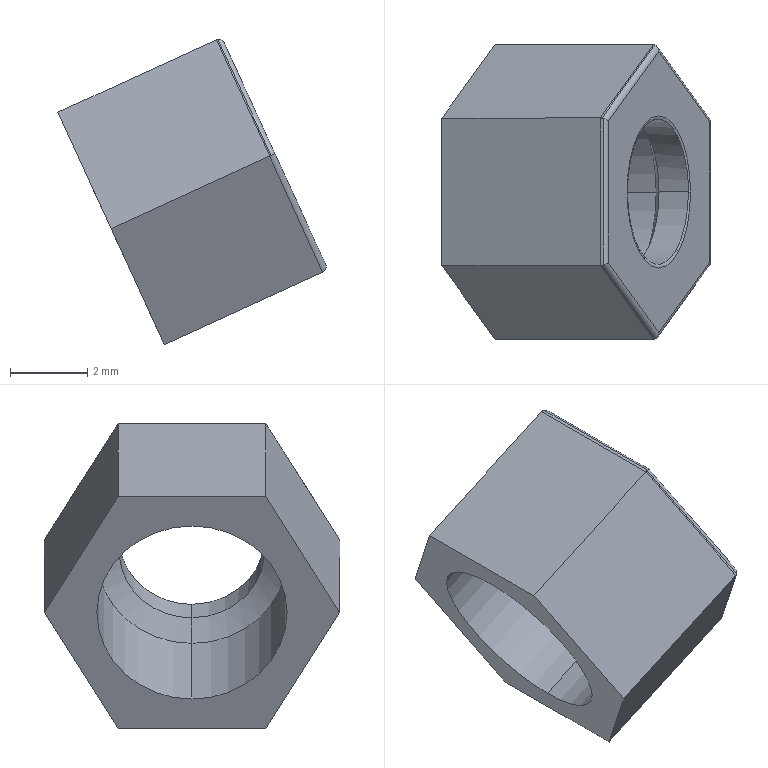Part | STEP file | 2026.6.15-Main Assembly图.sldasm-Part-206 | 1 solid | 25 faces | box 6.927 x 7.621 x 7.888 mm | volume 95.325 mm3 | cylinder 13 | plane 8 | torus 2 | cone 2 | commonest cylinder face diameters 0.3 x9 3.75 x2 4.913 x2
STEP:
#1=CARTESIAN_POINT('',(-1606.587,1438.31,3412.574));
#2=VERTEX_POINT('',#1);
#3=CARTESIAN_POINT('',(-1606.623,1438.304,3412.557));
#4=VERTEX_POINT('',#3);
#5=CARTESIAN_POINT('',(-1606.587,1438.31,3412.574));
#6=CARTESIAN_POINT('',(-1606.599,1438.306,3412.568));
#7=CARTESIAN_POINT('',(-1606.611,1438.304,3412.563));
#8=CARTESIAN_POINT('',(-1606.623,1438.304,3412.557));
#9=(BOUNDED_CURVE()B_SPLINE_CURVE(3,(#5,#6,#7,#8),.UNSPECIFIED.,.F.,.F.)B_SPLINE_CURVE_WITH_KNOTS((4,4),(0.8172,1.),.UNSPECIFIED.)CURVE()GEOMETRIC_REPRESENTATION_ITEM()RATIONAL_B_SPLINE_CURVE((0.9125,0.9351,0.9643,1.))REPRESENTATION_ITEM(''));
#10=EDGE_CURVE('',#2,#4,#9,.T.);
#11=ORIENTED_EDGE('',*,*,#10,.F.);
#12=CARTESIAN_POINT('',(-1607.958,1440.212,3415.569));
#13=VERTEX_POINT('',#12);
#14=CARTESIAN_POINT('',(-1609.333,1442.119,3418.572));
#15=DIRECTION('',(-0.3605,0.5,0.7874));
#16=VECTOR('',#15,1000.);
#17=LINE('',#14,#16);
#18=EDGE_CURVE('',#2,#13,#17,.T.);
#19=ORIENTED_EDGE('',*,*,#18,.T.);
#20=CARTESIAN_POINT('',(-1607.997,1440.209,3415.558));
#21=VERTEX_POINT('',#20);
#22=CARTESIAN_POINT('',(-1607.958,1440.212,3415.569));
#23=CARTESIAN_POINT('',(-1607.972,1440.21,3415.567));
#24=CARTESIAN_POINT('',(-1607.985,1440.209,3415.563));
#25=CARTESIAN_POINT('',(-1607.997,1440.209,3415.558));
#26=(BOUNDED_CURVE()B_SPLINE_CURVE(3,(#22,#23,#24,#25),.UNSPECIFIED.,.F.,.T.)B_SPLINE_CURVE_WITH_KNOTS((4,4),(0.8172,1.),.UNSPECIFIED.)CURVE()GEOMETRIC_REPRESENTATION_ITEM()RATIONAL_B_SPLINE_CURVE((0.9125,0.9351,0.9643,1.))REPRESENTATION_ITEM(''));
#27=EDGE_CURVE('',#13,#21,#26,.T.);
#28=ORIENTED_EDGE('',*,*,#27,.T.);
#29=CARTESIAN_POINT('',(-1606.623,1438.304,3412.557));
#30=DIRECTION('',(-0.3605,0.5,0.7874));
#31=VECTOR('',#30,1000.);
#32=LINE('',#29,#31);
#33=EDGE_CURVE('',#4,#21,#32,.T.);
#34=ORIENTED_EDGE('',*,*,#33,.F.);
#35=EDGE_LOOP('',(#11,#19,#28,#34));
#36=FACE_OUTER_BOUND('',#35,.T.);
#37=CARTESIAN_POINT('',(-1609.339,1442.244,3418.49));
#38=DIRECTION('',(-0.3605,0.5,0.7874));
#39=DIRECTION('',(0.04327,-0.8343,0.5496));
#40=AXIS2_PLACEMENT_3D('',#37,#38,#39);
#41=CYLINDRICAL_SURFACE('',#40,0.15);
#42=ADVANCED_FACE('',(#36),#41,.T.);
#43=CARTESIAN_POINT('',(-1607.923,1440.22,3415.571));
#44=VERTEX_POINT('',#43);
#45=CARTESIAN_POINT('',(-1607.923,1440.22,3415.571));
#46=CARTESIAN_POINT('',(-1607.934,1440.217,3415.572));
#47=CARTESIAN_POINT('',(-1607.946,1440.214,3415.571));
#48=CARTESIAN_POINT('',(-1607.958,1440.212,3415.569));
#49=(BOUNDED_CURVE()B_SPLINE_CURVE(3,(#45,#46,#47,#48),.UNSPECIFIED.,.F.,.T.)B_SPLINE_CURVE_WITH_KNOTS((4,4),(0.6686,0.8172),.UNSPECIFIED.)CURVE()GEOMETRIC_REPRESENTATION_ITEM()RATIONAL_B_SPLINE_CURVE((0.8702,0.88,0.8941,0.9125))REPRESENTATION_ITEM(''));
#50=EDGE_CURVE('',#44,#13,#49,.T.);
#51=ORIENTED_EDGE('',*,*,#50,.F.);
#52=CARTESIAN_POINT('',(-1607.923,1444.009,3415.571));
#53=VERTEX_POINT('',#52);
#54=CARTESIAN_POINT('',(-1607.923,1442.114,3415.571));
#55=DIRECTION('',(0.,1.,0.));
#56=VECTOR('',#55,1000.);
#57=LINE('',#54,#56);
#58=EDGE_CURVE('',#44,#53,#57,.T.);
#59=ORIENTED_EDGE('',*,*,#58,.T.);
#60=CARTESIAN_POINT('',(-1607.958,1444.016,3415.569));
#61=VERTEX_POINT('',#60);
#62=CARTESIAN_POINT('',(-1607.923,1444.009,3415.571));
#63=CARTESIAN_POINT('',(-1607.934,1444.012,3415.572));
#64=CARTESIAN_POINT('',(-1607.946,1444.015,3415.571));
#65=CARTESIAN_POINT('',(-1607.958,1444.016,3415.569));
#66=(BOUNDED_CURVE()B_SPLINE_CURVE(3,(#62,#63,#64,#65),.UNSPECIFIED.,.F.,.F.)B_SPLINE_CURVE_WITH_KNOTS((4,4),(0.6686,0.8172),.UNSPECIFIED.)CURVE()GEOMETRIC_REPRESENTATION_ITEM()RATIONAL_B_SPLINE_CURVE((0.8702,0.88,0.8941,0.9125))REPRESENTATION_ITEM(''));
#67=EDGE_CURVE('',#53,#61,#66,.T.);
#68=ORIENTED_EDGE('',*,*,#67,.T.);
#69=CARTESIAN_POINT('',(-1607.997,1444.02,3415.558));
#70=VERTEX_POINT('',#69);
#71=CARTESIAN_POINT('',(-1607.958,1444.016,3415.569));
#72=CARTESIAN_POINT('',(-1607.972,1444.019,3415.567));
#73=CARTESIAN_POINT('',(-1607.985,1444.02,3415.563));
#74=CARTESIAN_POINT('',(-1607.997,1444.02,3415.558));
#75=(BOUNDED_CURVE()B_SPLINE_CURVE(3,(#71,#72,#73,#74),.UNSPECIFIED.,.F.,.F.)B_SPLINE_CURVE_WITH_KNOTS((4,4),(0.8172,1.),.UNSPECIFIED.)CURVE()GEOMETRIC_REPRESENTATION_ITEM()RATIONAL_B_SPLINE_CURVE((0.9125,0.9351,0.9643,1.))REPRESENTATION_ITEM(''));
#76=EDGE_CURVE('',#61,#70,#75,.T.);
#77=ORIENTED_EDGE('',*,*,#76,.T.);
#78=CARTESIAN_POINT('',(-1607.997,1444.02,3415.558));
#79=DIRECTION('',(0.,1.,0.));
#80=VECTOR('',#79,1000.);
#81=LINE('',#78,#80);
#82=EDGE_CURVE('',#21,#70,#81,.T.);
#83=ORIENTED_EDGE('',*,*,#82,.F.);
#84=ORIENTED_EDGE('',*,*,#27,.F.);
#85=EDGE_LOOP('',(#51,#59,#68,#77,#83,#84));
#86=FACE_OUTER_BOUND('',#85,.T.);
#87=CARTESIAN_POINT('',(-1607.934,1442.114,3415.421));
#88=DIRECTION('',(0.,1.,0.));
#89=DIRECTION('',(0.0785,0.,0.9969));
#90=AXIS2_PLACEMENT_3D('',#87,#88,#89);
#91=CYLINDRICAL_SURFACE('',#90,0.15);
#92=ADVANCED_FACE('',(#86),#91,.T.);
#93=ORIENTED_EDGE('',*,*,#76,.F.);
#94=CARTESIAN_POINT('',(-1606.587,1445.918,3412.574));
#95=VERTEX_POINT('',#94);
#96=CARTESIAN_POINT('',(-1609.333,1442.11,3418.572));
#97=DIRECTION('',(0.3605,0.5,-0.7874));
#98=VECTOR('',#97,1000.);
#99=LINE('',#96,#98);
#100=EDGE_CURVE('',#61,#95,#99,.T.);
#101=ORIENTED_EDGE('',*,*,#100,.T.);
#102=CARTESIAN_POINT('',(-1606.623,1445.925,3412.557));
#103=VERTEX_POINT('',#102);
#104=CARTESIAN_POINT('',(-1606.623,1445.925,3412.557));
#105=CARTESIAN_POINT('',(-1606.611,1445.925,3412.563));
#106=CARTESIAN_POINT('',(-1606.599,1445.923,3412.568));
#107=CARTESIAN_POINT('',(-1606.587,1445.918,3412.574));
#108=(BOUNDED_CURVE()B_SPLINE_CURVE(3,(#104,#105,#106,#107),.UNSPECIFIED.,.F.,.T.)B_SPLINE_CURVE_WITH_KNOTS((4,4),(0.,0.1828),.UNSPECIFIED.)CURVE()GEOMETRIC_REPRESENTATION_ITEM()RATIONAL_B_SPLINE_CURVE((1.,0.9643,0.9351,0.9125))REPRESENTATION_ITEM(''));
#109=EDGE_CURVE('',#103,#95,#108,.T.);
#110=ORIENTED_EDGE('',*,*,#109,.F.);
#111=CARTESIAN_POINT('',(-1607.997,1444.02,3415.558));
#112=DIRECTION('',(0.3605,0.5,-0.7874));
#113=VECTOR('',#112,1000.);
#114=LINE('',#111,#113);
#115=EDGE_CURVE('',#70,#103,#114,.T.);
#116=ORIENTED_EDGE('',*,*,#115,.F.);
#117=EDGE_LOOP('',(#93,#101,#110,#116));
#118=FACE_OUTER_BOUND('',#117,.T.);
#119=CARTESIAN_POINT('',(-1609.339,1441.984,3418.49));
#120=DIRECTION('',(0.3605,0.5,-0.7874));
#121=DIRECTION('',(0.04327,0.8343,0.5496));
#122=AXIS2_PLACEMENT_3D('',#119,#120,#121);
#123=CYLINDRICAL_SURFACE('',#122,0.15);
#124=ADVANCED_FACE('',(#118),#123,.T.);
#125=CARTESIAN_POINT('',(-1605.175,1440.296,3409.756));
#126=VERTEX_POINT('',#125);
#127=CARTESIAN_POINT('',(-1606.487,1438.477,3412.62));
#128=VERTEX_POINT('',#127);
#129=CARTESIAN_POINT('',(-1607.892,1436.528,3415.688));
#130=DIRECTION('',(-0.3605,-0.5,0.7874));
#131=VECTOR('',#130,1000.);
#132=LINE('',#129,#131);
#133=EDGE_CURVE('',#126,#128,#132,.T.);
#134=ORIENTED_EDGE('',*,*,#133,.F.);
#135=CARTESIAN_POINT('',(-1605.175,1443.933,3409.756));
#136=VERTEX_POINT('',#135);
#137=CARTESIAN_POINT('',(-1605.175,1442.114,3409.756));
#138=DIRECTION('',(0.,-1.,0.));
#139=VECTOR('',#138,1000.);
#140=LINE('',#137,#139);
#141=EDGE_CURVE('',#136,#126,#140,.T.);
#142=ORIENTED_EDGE('',*,*,#141,.F.);
#143=CARTESIAN_POINT('',(-1606.487,1445.752,3412.62));
#144=VERTEX_POINT('',#143);
#145=CARTESIAN_POINT('',(-1607.892,1447.7,3415.688));
#146=DIRECTION('',(0.3605,-0.5,-0.7874));
#147=VECTOR('',#146,1000.);
#148=LINE('',#145,#147);
#149=EDGE_CURVE('',#144,#136,#148,.T.);
#150=ORIENTED_EDGE('',*,*,#149,.F.);
#151=CARTESIAN_POINT('',(-1607.798,1443.933,3415.484));
#152=VERTEX_POINT('',#151);
#153=CARTESIAN_POINT('',(-1609.203,1441.984,3418.552));
#154=DIRECTION('',(0.3605,0.5,-0.7874));
#155=VECTOR('',#154,1000.);
#156=LINE('',#153,#155);
#157=EDGE_CURVE('',#152,#144,#156,.T.);
#158=ORIENTED_EDGE('',*,*,#157,.F.);
#159=CARTESIAN_POINT('',(-1607.798,1440.296,3415.484));
#160=VERTEX_POINT('',#159);
#161=CARTESIAN_POINT('',(-1607.798,1442.114,3415.484));
#162=DIRECTION('',(0.,1.,0.));
#163=VECTOR('',#162,1000.);
#164=LINE('',#161,#163);
#165=EDGE_CURVE('',#160,#152,#164,.T.);
#166=ORIENTED_EDGE('',*,*,#165,.F.);
#167=CARTESIAN_POINT('',(-1609.203,1442.244,3418.552));
#168=DIRECTION('',(-0.3605,0.5,0.7874));
#169=VECTOR('',#168,1000.);
#170=LINE('',#167,#169);
#171=EDGE_CURVE('',#128,#160,#170,.T.);
#172=ORIENTED_EDGE('',*,*,#171,.F.);
#173=EDGE_LOOP('',(#134,#142,#150,#158,#166,#172));
#174=FACE_OUTER_BOUND('',#173,.T.);
#175=CARTESIAN_POINT('',(-1605.669,1442.114,3410.833));
#176=VERTEX_POINT('',#175);
#177=CARTESIAN_POINT('',(-1607.305,1442.114,3414.406));
#178=VERTEX_POINT('',#177);
#179=CARTESIAN_POINT('',(-1606.487,1442.114,3412.62));
#180=DIRECTION('',(0.9092,0.,0.4163));
#181=DIRECTION('',(0.4163,0.,-0.9092));
#182=AXIS2_PLACEMENT_3D('',#179,#180,#181);
#183=CIRCLE('',#182,1.965);
#184=EDGE_CURVE('',#176,#178,#183,.T.);
#185=ORIENTED_EDGE('',*,*,#184,.F.);
#186=CARTESIAN_POINT('',(-1606.487,1442.114,3412.62));
#187=DIRECTION('',(0.9092,0.,0.4163));
#188=DIRECTION('',(0.4163,0.,-0.9092));
#189=AXIS2_PLACEMENT_3D('',#186,#187,#188);
#190=CIRCLE('',#189,1.965);
#191=EDGE_CURVE('',#178,#176,#190,.T.);
#192=ORIENTED_EDGE('',*,*,#191,.F.);
#193=EDGE_LOOP('',(#185,#192));
#194=FACE_BOUND('',#193,.T.);
#195=CARTESIAN_POINT('',(-1609.234,1442.114,3418.621));
#196=DIRECTION('',(0.9092,0.,0.4163));
#197=DIRECTION('',(-0.4163,0.,0.9092));
#198=AXIS2_PLACEMENT_3D('',#195,#196,#197);
#199=PLANE('',#198);
#200=ADVANCED_FACE('',(#174,#194),#199,.T.);
#201=ORIENTED_EDGE('',*,*,#100,.F.);
#202=ORIENTED_EDGE('',*,*,#67,.F.);
#203=CARTESIAN_POINT('',(-1607.798,1443.933,3415.484));
#204=CARTESIAN_POINT('',(-1607.821,1443.964,3415.533));
#205=CARTESIAN_POINT('',(-1607.866,1443.993,3415.566));
#206=CARTESIAN_POINT('',(-1607.923,1444.009,3415.571));
#207=(BOUNDED_CURVE()B_SPLINE_CURVE(3,(#203,#204,#205,#206),.UNSPECIFIED.,.F.,.T.)B_SPLINE_CURVE_WITH_KNOTS((4,4),(0.,0.6686),.UNSPECIFIED.)CURVE()GEOMETRIC_REPRESENTATION_ITEM()RATIONAL_B_SPLINE_CURVE((1.,0.8695,0.8262,0.8702))REPRESENTATION_ITEM(''));
#208=EDGE_CURVE('',#152,#53,#207,.T.);
#209=ORIENTED_EDGE('',*,*,#208,.F.);
#210=ORIENTED_EDGE('',*,*,#157,.T.);
#211=CARTESIAN_POINT('',(-1606.587,1445.918,3412.574));
#212=CARTESIAN_POINT('',(-1606.524,1445.896,3412.603));
#213=CARTESIAN_POINT('',(-1606.487,1445.831,3412.62));
#214=CARTESIAN_POINT('',(-1606.487,1445.752,3412.62));
#215=(BOUNDED_CURVE()B_SPLINE_CURVE(3,(#211,#212,#213,#214),.UNSPECIFIED.,.F.,.F.)B_SPLINE_CURVE_WITH_KNOTS((4,4),(0.1828,1.),.UNSPECIFIED.)CURVE()GEOMETRIC_REPRESENTATION_ITEM()RATIONAL_B_SPLINE_CURVE((0.9125,0.8113,0.8404,1.))REPRESENTATION_ITEM(''));
#216=EDGE_CURVE('',#95,#144,#215,.T.);
#217=ORIENTED_EDGE('',*,*,#216,.F.);
#218=EDGE_LOOP('',(#201,#202,#209,#210,#217));
#219=FACE_OUTER_BOUND('',#218,.T.);
#220=CARTESIAN_POINT('',(-1609.339,1441.984,3418.49));
#221=DIRECTION('',(0.3605,0.5,-0.7874));
#222=DIRECTION('',(0.04327,0.8343,0.5496));
#223=AXIS2_PLACEMENT_3D('',#220,#221,#222);
#224=CYLINDRICAL_SURFACE('',#223,0.15);
#225=ADVANCED_FACE('',(#219),#224,.T.);
#226=ORIENTED_EDGE('',*,*,#58,.F.);
#227=CARTESIAN_POINT('',(-1607.798,1440.296,3415.484));
#228=CARTESIAN_POINT('',(-1607.821,1440.264,3415.533));
#229=CARTESIAN_POINT('',(-1607.866,1440.236,3415.566));
#230=CARTESIAN_POINT('',(-1607.923,1440.22,3415.571));
#231=(BOUNDED_CURVE()B_SPLINE_CURVE(3,(#227,#228,#229,#230),.UNSPECIFIED.,.F.,.F.)B_SPLINE_CURVE_WITH_KNOTS((4,4),(0.,0.6686),.UNSPECIFIED.)CURVE()GEOMETRIC_REPRESENTATION_ITEM()RATIONAL_B_SPLINE_CURVE((1.,0.8695,0.8262,0.8702))REPRESENTATION_ITEM(''));
#232=EDGE_CURVE('',#160,#44,#231,.T.);
#233=ORIENTED_EDGE('',*,*,#232,.F.);
#234=ORIENTED_EDGE('',*,*,#165,.T.);
#235=ORIENTED_EDGE('',*,*,#208,.T.);
#236=EDGE_LOOP('',(#226,#233,#234,#235));
#237=FACE_OUTER_BOUND('',#236,.T.);
#238=CARTESIAN_POINT('',(-1607.934,1442.114,3415.421));
#239=DIRECTION('',(0.,1.,0.));
#240=DIRECTION('',(0.0785,0.,0.9969));
#241=AXIS2_PLACEMENT_3D('',#238,#239,#240);
#242=CYLINDRICAL_SURFACE('',#241,0.15);
#243=ADVANCED_FACE('',(#237),#242,.T.);
#244=ORIENTED_EDGE('',*,*,#18,.F.);
#245=CARTESIAN_POINT('',(-1606.487,1438.477,3412.62));
#246=CARTESIAN_POINT('',(-1606.487,1438.398,3412.62));
#247=CARTESIAN_POINT('',(-1606.524,1438.332,3412.603));
#248=CARTESIAN_POINT('',(-1606.587,1438.31,3412.574));
#249=(BOUNDED_CURVE()B_SPLINE_CURVE(3,(#245,#246,#247,#248),.UNSPECIFIED.,.F.,.F.)B_SPLINE_CURVE_WITH_KNOTS((4,4),(0.,0.8172),.UNSPECIFIED.)CURVE()GEOMETRIC_REPRESENTATION_ITEM()RATIONAL_B_SPLINE_CURVE((1.,0.8404,0.8113,0.9125))REPRESENTATION_ITEM(''));
#250=EDGE_CURVE('',#128,#2,#249,.T.);
#251=ORIENTED_EDGE('',*,*,#250,.F.);
#252=ORIENTED_EDGE('',*,*,#171,.T.);
#253=ORIENTED_EDGE('',*,*,#232,.T.);
#254=ORIENTED_EDGE('',*,*,#50,.T.);
#255=EDGE_LOOP('',(#244,#251,#252,#253,#254));
#256=FACE_OUTER_BOUND('',#255,.T.);
#257=CARTESIAN_POINT('',(-1609.339,1442.244,3418.49));
#258=DIRECTION('',(-0.3605,0.5,0.7874));
#259=DIRECTION('',(0.04327,-0.8343,0.5496));
#260=AXIS2_PLACEMENT_3D('',#257,#258,#259);
#261=CYLINDRICAL_SURFACE('',#260,0.15);
#262=ADVANCED_FACE('',(#256),#261,.T.);
#263=CARTESIAN_POINT('',(-1605.249,1440.209,3409.557));
#264=VERTEX_POINT('',#263);
#265=CARTESIAN_POINT('',(-1605.175,1440.296,3409.756));
#266=CARTESIAN_POINT('',(-1605.139,1440.245,3409.676));
#267=CARTESIAN_POINT('',(-1605.169,1440.209,3409.593));
#268=CARTESIAN_POINT('',(-1605.249,1440.209,3409.557));
#269=(BOUNDED_CURVE()B_SPLINE_CURVE(3,(#265,#266,#267,#268),.UNSPECIFIED.,.F.,.F.)B_SPLINE_CURVE_WITH_KNOTS((4,4),(0.,1.),.UNSPECIFIED.)CURVE()GEOMETRIC_REPRESENTATION_ITEM()RATIONAL_B_SPLINE_CURVE((1.,0.8047,0.8047,1.))REPRESENTATION_ITEM(''));
#270=EDGE_CURVE('',#126,#264,#269,.T.);
#271=ORIENTED_EDGE('',*,*,#270,.F.);
#272=ORIENTED_EDGE('',*,*,#133,.T.);
#273=ORIENTED_EDGE('',*,*,#250,.T.);
#274=ORIENTED_EDGE('',*,*,#10,.T.);
#275=CARTESIAN_POINT('',(-1605.249,1440.209,3409.557));
#276=DIRECTION('',(-0.3605,-0.5,0.7874));
#277=VECTOR('',#276,1000.);
#278=LINE('',#275,#277);
#279=EDGE_CURVE('',#264,#4,#278,.T.);
#280=ORIENTED_EDGE('',*,*,#279,.F.);
#281=EDGE_LOOP('',(#271,#272,#273,#274,#280));
#282=FACE_OUTER_BOUND('',#281,.T.);
#283=CARTESIAN_POINT('',(-1608.028,1436.528,3415.626));
#284=DIRECTION('',(-0.3605,-0.5,0.7874));
#285=DIRECTION('',(-0.04327,-0.8343,-0.5496));
#286=AXIS2_PLACEMENT_3D('',#283,#284,#285);
#287=CYLINDRICAL_SURFACE('',#286,0.15);
#288=ADVANCED_FACE('',(#282),#287,.T.);
#289=CARTESIAN_POINT('',(-1605.249,1444.02,3409.557));
#290=VERTEX_POINT('',#289);
#291=CARTESIAN_POINT('',(-1605.175,1443.933,3409.756));
#292=CARTESIAN_POINT('',(-1605.139,1443.984,3409.676));
#293=CARTESIAN_POINT('',(-1605.169,1444.02,3409.593));
#294=CARTESIAN_POINT('',(-1605.249,1444.02,3409.557));
#295=(BOUNDED_CURVE()B_SPLINE_CURVE(3,(#291,#292,#293,#294),.UNSPECIFIED.,.F.,.F.)B_SPLINE_CURVE_WITH_KNOTS((4,4),(0.,1.),.UNSPECIFIED.)CURVE()GEOMETRIC_REPRESENTATION_ITEM()RATIONAL_B_SPLINE_CURVE((1.,0.8047,0.8047,1.))REPRESENTATION_ITEM(''));
#296=EDGE_CURVE('',#136,#290,#295,.T.);
#297=ORIENTED_EDGE('',*,*,#296,.F.);
#298=ORIENTED_EDGE('',*,*,#141,.T.);
#299=ORIENTED_EDGE('',*,*,#270,.T.);
#300=CARTESIAN_POINT('',(-1605.249,1444.02,3409.557));
#301=DIRECTION('',(0.,-1.,0.));
#302=VECTOR('',#301,1000.);
#303=LINE('',#300,#302);
#304=EDGE_CURVE('',#290,#264,#303,.T.);
#305=ORIENTED_EDGE('',*,*,#304,.F.);
#306=EDGE_LOOP('',(#297,#298,#299,#305));
#307=FACE_OUTER_BOUND('',#306,.T.);
#308=CARTESIAN_POINT('',(-1605.312,1442.114,3409.693));
#309=DIRECTION('',(0.,-1.,0.));
#310=DIRECTION('',(-0.0785,0.,-0.9969));
#311=AXIS2_PLACEMENT_3D('',#308,#309,#310);
#312=CYLINDRICAL_SURFACE('',#311,0.15);
#313=ADVANCED_FACE('',(#307),#312,.T.);
#314=ORIENTED_EDGE('',*,*,#296,.T.);
#315=CARTESIAN_POINT('',(-1606.623,1445.925,3412.557));
#316=DIRECTION('',(0.3605,-0.5,-0.7874));
#317=VECTOR('',#316,1000.);
#318=LINE('',#315,#317);
#319=EDGE_CURVE('',#103,#290,#318,.T.);
#320=ORIENTED_EDGE('',*,*,#319,.F.);
#321=ORIENTED_EDGE('',*,*,#109,.T.);
#322=ORIENTED_EDGE('',*,*,#216,.T.);
#323=ORIENTED_EDGE('',*,*,#149,.T.);
#324=EDGE_LOOP('',(#314,#320,#321,#322,#323));
#325=FACE_OUTER_BOUND('',#324,.T.);
#326=CARTESIAN_POINT('',(-1608.028,1447.7,3415.626));
#327=DIRECTION('',(0.3605,-0.5,-0.7874));
#328=DIRECTION('',(-0.04327,0.8343,-0.5496));
#329=AXIS2_PLACEMENT_3D('',#326,#327,#328);
#330=CYLINDRICAL_SURFACE('',#329,0.15);
#331=ADVANCED_FACE('',(#325),#330,.T.);
#332=CARTESIAN_POINT('',(-1607.298,1442.114,3414.299));
#333=VERTEX_POINT('',#332);
#334=CARTESIAN_POINT('',(-1607.441,1442.114,3414.344));
#335=DIRECTION('',(0.,1.,0.));
#336=DIRECTION('',(0.9969,0.,-0.0785));
#337=AXIS2_PLACEMENT_3D('',#334,#335,#336);
#338=CIRCLE('',#337,0.15);
#339=EDGE_CURVE('',#178,#333,#338,.T.);
#340=ORIENTED_EDGE('',*,*,#339,.F.);
#341=ORIENTED_EDGE('',*,*,#191,.T.);
#342=CARTESIAN_POINT('',(-1605.722,1442.114,3410.896));
#343=VERTEX_POINT('',#342);
#344=CARTESIAN_POINT('',(-1605.805,1442.114,3410.771));
#345=DIRECTION('',(0.,-1.,0.));
#346=DIRECTION('',(-0.9969,0.,0.0785));
#347=AXIS2_PLACEMENT_3D('',#344,#345,#346);
#348=CIRCLE('',#347,0.15);
#349=EDGE_CURVE('',#176,#343,#348,.T.);
#350=ORIENTED_EDGE('',*,*,#349,.T.);
#351=CARTESIAN_POINT('',(-1605.722,1442.114,3410.896));
#352=CARTESIAN_POINT('',(-1605.723,1441.867,3410.896));
#353=CARTESIAN_POINT('',(-1605.744,1441.622,3410.941));
#354=CARTESIAN_POINT('',(-1605.804,1441.284,3411.069));
#355=CARTESIAN_POINT('',(-1605.829,1441.174,3411.123));
#356=CARTESIAN_POINT('',(-1605.886,1440.971,3411.246));
#357=CARTESIAN_POINT('',(-1605.919,1440.877,3411.316));
#358=CARTESIAN_POINT('',(-1606.029,1440.616,3411.553));
#359=CARTESIAN_POINT('',(-1606.115,1440.479,3411.74));
#360=CARTESIAN_POINT('',(-1606.259,1440.338,3412.051));
#361=CARTESIAN_POINT('',(-1606.308,1440.302,3412.157));
#362=CARTESIAN_POINT('',(-1606.409,1440.255,3412.374));
#363=CARTESIAN_POINT('',(-1606.461,1440.243,3412.486));
#364=CARTESIAN_POINT('',(-1606.564,1440.243,3412.709));
#365=CARTESIAN_POINT('',(-1606.615,1440.255,3412.819));
#366=CARTESIAN_POINT('',(-1606.716,1440.303,3413.037));
#367=CARTESIAN_POINT('',(-1606.766,1440.339,3413.145));
#368=CARTESIAN_POINT('',(-1606.908,1440.479,3413.452));
#369=CARTESIAN_POINT('',(-1606.996,1440.618,3413.641));
#370=CARTESIAN_POINT('',(-1607.141,1440.963,3413.955));
#371=CARTESIAN_POINT('',(-1607.199,1441.171,3414.082));
#372=CARTESIAN_POINT('',(-1607.258,1441.509,3414.21));
#373=CARTESIAN_POINT('',(-1607.273,1441.629,3414.243));
#374=CARTESIAN_POINT('',(-1607.293,1441.869,3414.287));
#375=CARTESIAN_POINT('',(-1607.298,1441.991,3414.298));
#376=CARTESIAN_POINT('',(-1607.298,1442.114,3414.299));
#377=B_SPLINE_CURVE_WITH_KNOTS('',3,(#351,#352,#353,#354,#355,#356,#357,#358,#359,#360,#361,#362,#363,#364,#365,#366,#367,#368,#369,#370,#371,#372,#373,#374,#375,#376),.UNSPECIFIED.,.F.,.F.,(4,2,2,2,2,2,2,2,2,2,2,2,4),(0.,0.0007396,0.001109,0.001479,0.002219,0.002589,0.002958,0.003328,0.003698,0.004438,0.005177,0.005547,0.005917),.UNSPECIFIED.);
#378=EDGE_CURVE('',#343,#333,#377,.T.);
#379=ORIENTED_EDGE('',*,*,#378,.T.);
#380=EDGE_LOOP('',(#340,#341,#350,#379));
#381=FACE_OUTER_BOUND('',#380,.T.);
#382=CARTESIAN_POINT('',(-1606.623,1442.114,3412.557));
#383=DIRECTION('',(0.9092,0.,0.4163));
#384=DIRECTION('',(-0.4163,0.,0.9092));
#385=AXIS2_PLACEMENT_3D('',#382,#383,#384);
#386=TOROIDAL_SURFACE('',#385,1.965,0.15);
#387=ADVANCED_FACE('',(#381),#386,.T.);
#388=CARTESIAN_POINT('',(-1612.088,1444.02,3413.684));
#389=VERTEX_POINT('',#388);
#390=CARTESIAN_POINT('',(-1612.088,1444.02,3413.684));
#391=DIRECTION('',(-0.9092,0.,-0.4163));
#392=VECTOR('',#391,1000.);
#393=LINE('',#390,#392);
#394=EDGE_CURVE('',#70,#389,#393,.T.);
#395=ORIENTED_EDGE('',*,*,#394,.F.);
#396=ORIENTED_EDGE('',*,*,#115,.T.);
#397=CARTESIAN_POINT('',(-1610.715,1445.925,3410.684));
#398=VERTEX_POINT('',#397);
#399=CARTESIAN_POINT('',(-1610.715,1445.925,3410.684));
#400=DIRECTION('',(0.9092,0.,0.4163));
#401=VECTOR('',#400,1000.);
#402=LINE('',#399,#401);
#403=EDGE_CURVE('',#398,#103,#402,.T.);
#404=ORIENTED_EDGE('',*,*,#403,.F.);
#405=CARTESIAN_POINT('',(-1610.715,1445.925,3410.684));
#406=DIRECTION('',(-0.3605,-0.5,0.7874));
#407=VECTOR('',#406,1000.);
#408=LINE('',#405,#407);
#409=EDGE_CURVE('',#398,#389,#408,.T.);
#410=ORIENTED_EDGE('',*,*,#409,.T.);
#411=EDGE_LOOP('',(#395,#396,#404,#410));
#412=FACE_OUTER_BOUND('',#411,.T.);
#413=CARTESIAN_POINT('',(-1610.715,1445.925,3410.684));
#414=DIRECTION('',(-0.2081,0.866,0.4546));
#415=DIRECTION('',(-0.9092,0.,-0.4163));
#416=AXIS2_PLACEMENT_3D('',#413,#414,#415);
#417=PLANE('',#416);
#418=ADVANCED_FACE('',(#412),#417,.T.);
#419=CARTESIAN_POINT('',(-1612.088,1440.209,3413.684));
#420=VERTEX_POINT('',#419);
#421=CARTESIAN_POINT('',(-1607.997,1440.209,3415.558));
#422=DIRECTION('',(-0.9092,0.,-0.4163));
#423=VECTOR('',#422,1000.);
#424=LINE('',#421,#423);
#425=EDGE_CURVE('',#21,#420,#424,.T.);
#426=ORIENTED_EDGE('',*,*,#425,.F.);
#427=ORIENTED_EDGE('',*,*,#82,.T.);
#428=ORIENTED_EDGE('',*,*,#394,.T.);
#429=CARTESIAN_POINT('',(-1612.088,1442.114,3413.684));
#430=DIRECTION('',(0.,-1.,0.));
#431=VECTOR('',#430,1000.);
#432=LINE('',#429,#431);
#433=EDGE_CURVE('',#389,#420,#432,.T.);
#434=ORIENTED_EDGE('',*,*,#433,.T.);
#435=EDGE_LOOP('',(#426,#427,#428,#434));
#436=FACE_OUTER_BOUND('',#435,.T.);
#437=CARTESIAN_POINT('',(-1612.088,1444.02,3413.684));
#438=DIRECTION('',(-0.4163,0.,0.9092));
#439=DIRECTION('',(0.,1.,0.));
#440=AXIS2_PLACEMENT_3D('',#437,#438,#439);
#441=PLANE('',#440);
#442=ADVANCED_FACE('',(#436),#441,.T.);
#443=CARTESIAN_POINT('',(-1610.715,1438.304,3410.684));
#444=VERTEX_POINT('',#443);
#445=CARTESIAN_POINT('',(-1606.623,1438.304,3412.557));
#446=DIRECTION('',(-0.9092,0.,-0.4163));
#447=VECTOR('',#446,1000.);
#448=LINE('',#445,#447);
#449=EDGE_CURVE('',#4,#444,#448,.T.);
#450=ORIENTED_EDGE('',*,*,#449,.F.);
#451=ORIENTED_EDGE('',*,*,#33,.T.);
#452=ORIENTED_EDGE('',*,*,#425,.T.);
#453=CARTESIAN_POINT('',(-1612.088,1440.209,3413.684));
#454=DIRECTION('',(0.3605,-0.5,-0.7874));
#455=VECTOR('',#454,1000.);
#456=LINE('',#453,#455);
#457=EDGE_CURVE('',#420,#444,#456,.T.);
#458=ORIENTED_EDGE('',*,*,#457,.T.);
#459=EDGE_LOOP('',(#450,#451,#452,#458));
#460=FACE_OUTER_BOUND('',#459,.T.);
#461=CARTESIAN_POINT('',(-1612.088,1440.209,3413.684));
#462=DIRECTION('',(-0.2081,-0.866,0.4546));
#463=DIRECTION('',(0.,-0.4648,-0.8854));
#464=AXIS2_PLACEMENT_3D('',#461,#462,#463);
#465=PLANE('',#464);
#466=ADVANCED_FACE('',(#460),#465,.T.);
#467=CARTESIAN_POINT('',(-1609.341,1440.209,3407.683));
#468=VERTEX_POINT('',#467);
#469=CARTESIAN_POINT('',(-1609.341,1440.209,3407.683));
#470=DIRECTION('',(-0.9092,0.,-0.4163));
#471=VECTOR('',#470,1000.);
#472=LINE('',#469,#471);
#473=EDGE_CURVE('',#264,#468,#472,.T.);
#474=ORIENTED_EDGE('',*,*,#473,.F.);
#475=ORIENTED_EDGE('',*,*,#279,.T.);
#476=ORIENTED_EDGE('',*,*,#449,.T.);
#477=CARTESIAN_POINT('',(-1610.715,1438.304,3410.684));
#478=DIRECTION('',(0.3605,0.5,-0.7874));
#479=VECTOR('',#478,1000.);
#480=LINE('',#477,#479);
#481=EDGE_CURVE('',#444,#468,#480,.T.);
#482=ORIENTED_EDGE('',*,*,#481,.T.);
#483=EDGE_LOOP('',(#474,#475,#476,#482));
#484=FACE_OUTER_BOUND('',#483,.T.);
#485=CARTESIAN_POINT('',(-1609.341,1440.209,3407.683));
#486=DIRECTION('',(0.2081,-0.866,-0.4546));
#487=DIRECTION('',(-0.9723,-0.2337,0.));
#488=AXIS2_PLACEMENT_3D('',#485,#486,#487);
#489=PLANE('',#488);
#490=ADVANCED_FACE('',(#484),#489,.T.);
#491=CARTESIAN_POINT('',(-1609.341,1444.02,3407.683));
#492=VERTEX_POINT('',#491);
#493=CARTESIAN_POINT('',(-1605.249,1444.02,3409.557));
#494=DIRECTION('',(-0.9092,0.,-0.4163));
#495=VECTOR('',#494,1000.);
#496=LINE('',#493,#495);
#497=EDGE_CURVE('',#290,#492,#496,.T.);
#498=ORIENTED_EDGE('',*,*,#497,.F.);
#499=ORIENTED_EDGE('',*,*,#304,.T.);
#500=ORIENTED_EDGE('',*,*,#473,.T.);
#501=CARTESIAN_POINT('',(-1609.341,1442.114,3407.683));
#502=DIRECTION('',(0.,1.,0.));
#503=VECTOR('',#502,1000.);
#504=LINE('',#501,#503);
#505=EDGE_CURVE('',#468,#492,#504,.T.);
#506=ORIENTED_EDGE('',*,*,#505,.T.);
#507=EDGE_LOOP('',(#498,#499,#500,#506));
#508=FACE_OUTER_BOUND('',#507,.T.);
#509=CARTESIAN_POINT('',(-1609.341,1444.02,3407.683));
#510=DIRECTION('',(0.4163,0.,-0.9092));
#511=DIRECTION('',(0.,-1.,0.));
#512=AXIS2_PLACEMENT_3D('',#509,#510,#511);
#513=PLANE('',#512);
#514=ADVANCED_FACE('',(#508),#513,.T.);
#515=ORIENTED_EDGE('',*,*,#403,.T.);
#516=ORIENTED_EDGE('',*,*,#319,.T.);
#517=ORIENTED_EDGE('',*,*,#497,.T.);
#518=CARTESIAN_POINT('',(-1609.341,1444.02,3407.683));
#519=DIRECTION('',(-0.3605,0.5,0.7874));
#520=VECTOR('',#519,1000.);
#521=LINE('',#518,#520);
#522=EDGE_CURVE('',#492,#398,#521,.T.);
#523=ORIENTED_EDGE('',*,*,#522,.T.);
#524=EDGE_LOOP('',(#515,#516,#517,#523));
#525=FACE_OUTER_BOUND('',#524,.T.);
#526=CARTESIAN_POINT('',(-1609.341,1444.02,3407.683));
#527=DIRECTION('',(0.2081,0.866,-0.4546));
#528=DIRECTION('',(0.9092,0.,0.4163));
#529=AXIS2_PLACEMENT_3D('',#526,#527,#528);
#530=PLANE('',#529);
#531=ADVANCED_FACE('',(#525),#530,.T.);
#532=CARTESIAN_POINT('',(-1606.481,1442.118,3410.548));
#533=VERTEX_POINT('',#532);
#534=CARTESIAN_POINT('',(-1605.722,1442.118,3410.896));
#535=VERTEX_POINT('',#534);
#536=CARTESIAN_POINT('',(-1638.843,1442.118,3395.732));
#537=DIRECTION('',(0.9092,0.,0.4163));
#538=VECTOR('',#537,1000.);
#539=LINE('',#536,#538);
#540=EDGE_CURVE('',#533,#535,#539,.T.);
#541=ORIENTED_EDGE('',*,*,#540,.T.);
#542=CARTESIAN_POINT('',(-1607.298,1442.118,3414.299));
#543=VERTEX_POINT('',#542);
#544=CARTESIAN_POINT('',(-1607.298,1442.118,3414.299));
#545=CARTESIAN_POINT('',(-1607.298,1442.365,3414.299));
#546=CARTESIAN_POINT('',(-1607.276,1442.611,3414.254));
#547=CARTESIAN_POINT('',(-1607.217,1442.95,3414.127));
#548=CARTESIAN_POINT('',(-1607.192,1443.06,3414.073));
#549=CARTESIAN_POINT('',(-1607.134,1443.263,3413.95));
#550=CARTESIAN_POINT('',(-1607.101,1443.358,3413.88));
#551=CARTESIAN_POINT('',(-1606.991,1443.619,3413.643));
#552=CARTESIAN_POINT('',(-1606.904,1443.756,3413.456));
#553=CARTESIAN_POINT('',(-1606.76,1443.898,3413.145));
#554=CARTESIAN_POINT('',(-1606.711,1443.933,3413.039));
#555=CARTESIAN_POINT('',(-1606.61,1443.981,3412.821));
#556=CARTESIAN_POINT('',(-1606.558,1443.993,3412.709));
#557=CARTESIAN_POINT('',(-1606.455,1443.993,3412.486));
#558=CARTESIAN_POINT('',(-1606.404,1443.981,3412.376));
#559=CARTESIAN_POINT('',(-1606.303,1443.933,3412.157));
#560=CARTESIAN_POINT('',(-1606.253,1443.897,3412.049));
#561=CARTESIAN_POINT('',(-1606.111,1443.756,3411.742));
#562=CARTESIAN_POINT('',(-1606.024,1443.617,3411.552));
#563=CARTESIAN_POINT('',(-1605.915,1443.358,3411.317));
#564=CARTESIAN_POINT('',(-1605.882,1443.262,3411.245));
#565=CARTESIAN_POINT('',(-1605.825,1443.057,3411.121));
#566=CARTESIAN_POINT('',(-1605.801,1442.95,3411.069));
#567=CARTESIAN_POINT('',(-1605.762,1442.724,3410.983));
#568=CARTESIAN_POINT('',(-1605.747,1442.604,3410.95));
#569=CARTESIAN_POINT('',(-1605.727,1442.364,3410.907));
#570=CARTESIAN_POINT('',(-1605.722,1442.242,3410.896));
#571=CARTESIAN_POINT('',(-1605.722,1442.118,3410.896));
#572=B_SPLINE_CURVE_WITH_KNOTS('',3,(#544,#545,#546,#547,#548,#549,#550,#551,#552,#553,#554,#555,#556,#557,#558,#559,#560,#561,#562,#563,#564,#565,#566,#567,#568,#569,#570,#571),.UNSPECIFIED.,.F.,.F.,(4,2,2,2,2,2,2,2,2,2,2,2,2,4),(0.,0.0007405,0.001111,0.001481,0.002221,0.002592,0.002962,0.003332,0.003702,0.004443,0.004813,0.005183,0.005554,0.005924),.UNSPECIFIED.);
#573=EDGE_CURVE('',#543,#535,#572,.T.);
#574=ORIENTED_EDGE('',*,*,#573,.F.);
#575=CARTESIAN_POINT('',(-1608.03,1442.118,3413.963));
#576=VERTEX_POINT('',#575);
#577=CARTESIAN_POINT('',(-1640.404,1442.118,3399.141));
#578=DIRECTION('',(0.9092,0.,0.4163));
#579=VECTOR('',#578,1000.);
#580=LINE('',#577,#579);
#581=EDGE_CURVE('',#576,#543,#580,.T.);
#582=ORIENTED_EDGE('',*,*,#581,.F.);
#583=CARTESIAN_POINT('',(-1608.03,1442.118,3413.963));
#584=CARTESIAN_POINT('',(-1608.031,1442.242,3413.963));
#585=CARTESIAN_POINT('',(-1608.026,1442.364,3413.952));
#586=CARTESIAN_POINT('',(-1608.006,1442.603,3413.909));
#587=CARTESIAN_POINT('',(-1607.991,1442.722,3413.876));
#588=CARTESIAN_POINT('',(-1607.953,1442.949,3413.79));
#589=CARTESIAN_POINT('',(-1607.929,1443.057,3413.738));
#590=CARTESIAN_POINT('',(-1607.873,1443.261,3413.614));
#591=CARTESIAN_POINT('',(-1607.841,1443.357,3413.541));
#592=CARTESIAN_POINT('',(-1607.734,1443.617,3413.305));
#593=CARTESIAN_POINT('',(-1607.647,1443.756,3413.114));
#594=CARTESIAN_POINT('',(-1607.461,1443.943,3412.704));
#595=CARTESIAN_POINT('',(-1607.359,1443.993,3412.479));
#596=CARTESIAN_POINT('',(-1607.208,1443.993,3412.145));
#597=CARTESIAN_POINT('',(-1607.156,1443.981,3412.032));
#598=CARTESIAN_POINT('',(-1607.057,1443.933,3411.813));
#599=CARTESIAN_POINT('',(-1607.009,1443.898,3411.706));
#600=CARTESIAN_POINT('',(-1606.915,1443.804,3411.5));
#601=CARTESIAN_POINT('',(-1606.869,1443.745,3411.4));
#602=CARTESIAN_POINT('',(-1606.785,1443.61,3411.215));
#603=CARTESIAN_POINT('',(-1606.746,1443.532,3411.128));
#604=CARTESIAN_POINT('',(-1606.673,1443.357,3410.969));
#605=CARTESIAN_POINT('',(-1606.641,1443.262,3410.898));
#606=CARTESIAN_POINT('',(-1606.585,1443.059,3410.775));
#607=CARTESIAN_POINT('',(-1606.56,1442.95,3410.721));
#608=CARTESIAN_POINT('',(-1606.521,1442.723,3410.636));
#609=CARTESIAN_POINT('',(-1606.506,1442.606,3410.603));
#610=CARTESIAN_POINT('',(-1606.486,1442.366,3410.56));
#611=CARTESIAN_POINT('',(-1606.481,1442.242,3410.548));
#612=CARTESIAN_POINT('',(-1606.481,1442.118,3410.548));
#613=B_SPLINE_CURVE_WITH_KNOTS('',3,(#583,#584,#585,#586,#587,#588,#589,#590,#591,#592,#593,#594,#595,#596,#597,#598,#599,#600,#601,#602,#603,#604,#605,#606,#607,#608,#609,#610,#611,#612),.UNSPECIFIED.,.F.,.F.,(4,2,2,2,2,2,2,2,2,2,2,2,2,2,4),(0.,0.0003663,0.0007326,0.001099,0.001465,0.002198,0.00293,0.003297,0.003663,0.004029,0.004396,0.004762,0.005128,0.005495,0.005861),.UNSPECIFIED.);
#614=EDGE_CURVE('',#576,#533,#613,.T.);
#615=ORIENTED_EDGE('',*,*,#614,.T.);
#616=EDGE_LOOP('',(#541,#574,#582,#615));
#617=FACE_OUTER_BOUND('',#616,.T.);
#618=CARTESIAN_POINT('',(-1639.624,1442.118,3397.437));
#619=DIRECTION('',(-0.9092,0.,-0.4163));
#620=DIRECTION('',(0.4163,0.,-0.9092));
#621=AXIS2_PLACEMENT_3D('',#618,#619,#620);
#622=CYLINDRICAL_SURFACE('',#621,1.875);
#623=ADVANCED_FACE('',(#617),#622,.F.);
#624=ORIENTED_EDGE('',*,*,#505,.F.);
#625=ORIENTED_EDGE('',*,*,#481,.F.);
#626=ORIENTED_EDGE('',*,*,#457,.F.);
#627=ORIENTED_EDGE('',*,*,#433,.F.);
#628=ORIENTED_EDGE('',*,*,#409,.F.);
#629=ORIENTED_EDGE('',*,*,#522,.F.);
#630=EDGE_LOOP('',(#624,#625,#626,#627,#628,#629));
#631=FACE_OUTER_BOUND('',#630,.T.);
#632=CARTESIAN_POINT('',(-1611.737,1442.114,3412.917));
#633=VERTEX_POINT('',#632);
#634=CARTESIAN_POINT('',(-1609.692,1442.114,3408.45));
#635=VERTEX_POINT('',#634);
#636=CARTESIAN_POINT('',(-1610.715,1442.114,3410.684));
#637=DIRECTION('',(0.9092,0.,0.4163));
#638=DIRECTION('',(-0.4163,0.,0.9092));
#639=AXIS2_PLACEMENT_3D('',#636,#637,#638);
#640=CIRCLE('',#639,2.456);
#641=EDGE_CURVE('',#633,#635,#640,.T.);
#642=ORIENTED_EDGE('',*,*,#641,.T.);
#643=CARTESIAN_POINT('',(-1610.715,1442.114,3410.684));
#644=DIRECTION('',(0.9092,0.,0.4163));
#645=DIRECTION('',(-0.4163,0.,0.9092));
#646=AXIS2_PLACEMENT_3D('',#643,#644,#645);
#647=CIRCLE('',#646,2.456);
#648=EDGE_CURVE('',#635,#633,#647,.T.);
#649=ORIENTED_EDGE('',*,*,#648,.T.);
#650=EDGE_LOOP('',(#642,#649));
#651=FACE_BOUND('',#650,.T.);
#652=CARTESIAN_POINT('',(-1613.462,1442.114,3416.685));
#653=DIRECTION('',(0.9092,0.,0.4163));
#654=DIRECTION('',(-0.4163,0.,0.9092));
#655=AXIS2_PLACEMENT_3D('',#652,#653,#654);
#656=PLANE('',#655);
#657=ADVANCED_FACE('',(#631,#651),#656,.F.);
#658=CARTESIAN_POINT('',(-1606.555,1442.114,3409.887));
#659=VERTEX_POINT('',#658);
#660=CARTESIAN_POINT('',(-1606.481,1442.114,3410.548));
#661=VERTEX_POINT('',#660);
#662=CARTESIAN_POINT('',(-1606.555,1442.114,3409.887));
#663=DIRECTION('',(0.1115,0.,0.9938));
#664=VECTOR('',#663,1000.);
#665=LINE('',#662,#664);
#666=EDGE_CURVE('',#659,#661,#665,.T.);
#667=ORIENTED_EDGE('',*,*,#666,.T.);
#668=CARTESIAN_POINT('',(-1606.481,1442.114,3410.548));
#669=CARTESIAN_POINT('',(-1606.481,1442.115,3410.548));
#670=CARTESIAN_POINT('',(-1606.481,1442.117,3410.548));
#671=CARTESIAN_POINT('',(-1606.481,1442.118,3410.548));
#672=B_SPLINE_CURVE_WITH_KNOTS('',3,(#668,#669,#670,#671),.UNSPECIFIED.,.F.,.F.,(4,4),(0.,1.),.UNSPECIFIED.);
#673=EDGE_CURVE('',#661,#533,#672,.T.);
#674=ORIENTED_EDGE('',*,*,#673,.T.);
#675=ORIENTED_EDGE('',*,*,#614,.F.);
#676=CARTESIAN_POINT('',(-1608.03,1442.114,3413.963));
#677=VERTEX_POINT('',#676);
#678=CARTESIAN_POINT('',(-1608.03,1442.118,3413.963));
#679=CARTESIAN_POINT('',(-1608.03,1442.117,3413.963));
#680=CARTESIAN_POINT('',(-1608.03,1442.115,3413.963));
#681=CARTESIAN_POINT('',(-1608.03,1442.114,3413.963));
#682=B_SPLINE_CURVE_WITH_KNOTS('',3,(#678,#679,#680,#681),.UNSPECIFIED.,.F.,.F.,(4,4),(0.,1.),.UNSPECIFIED.);
#683=EDGE_CURVE('',#576,#677,#682,.T.);
#684=ORIENTED_EDGE('',*,*,#683,.T.);
#685=CARTESIAN_POINT('',(-1608.6,1442.114,3414.354));
#686=VERTEX_POINT('',#685);
#687=CARTESIAN_POINT('',(-1608.6,1442.114,3414.354));
#688=DIRECTION('',(0.8251,0.,-0.565));
#689=VECTOR('',#688,1000.);
#690=LINE('',#687,#689);
#691=EDGE_CURVE('',#686,#677,#690,.T.);
#692=ORIENTED_EDGE('',*,*,#691,.F.);
#693=CARTESIAN_POINT('',(-1607.578,1442.114,3412.12));
#694=DIRECTION('',(-0.9092,0.,-0.4163));
#695=DIRECTION('',(-0.4163,0.,0.9092));
#696=AXIS2_PLACEMENT_3D('',#693,#694,#695);
#697=CIRCLE('',#696,2.456);
#698=EDGE_CURVE('',#686,#659,#697,.T.);
#699=ORIENTED_EDGE('',*,*,#698,.T.);
#700=EDGE_LOOP('',(#667,#674,#675,#684,#692,#699));
#701=FACE_OUTER_BOUND('',#700,.T.);
#702=CARTESIAN_POINT('',(-1607.578,1442.114,3412.12));
#703=DIRECTION('',(-0.9092,0.,-0.4163));
#704=DIRECTION('',(0.4163,0.,-0.9092));
#705=AXIS2_PLACEMENT_3D('',#702,#703,#704);
#706=CONICAL_SURFACE('',#705,2.456,1.03);
#707=ADVANCED_FACE('',(#701),#706,.F.);
#708=CARTESIAN_POINT('',(-1609.692,1442.114,3408.45));
#709=DIRECTION('',(0.9092,0.,0.4163));
#710=VECTOR('',#709,1000.);
#711=LINE('',#708,#710);
#712=EDGE_CURVE('',#635,#659,#711,.T.);
#713=ORIENTED_EDGE('',*,*,#712,.T.);
#714=ORIENTED_EDGE('',*,*,#698,.F.);
#715=CARTESIAN_POINT('',(-1611.737,1442.114,3412.917));
#716=DIRECTION('',(0.9092,0.,0.4163));
#717=VECTOR('',#716,1000.);
#718=LINE('',#715,#717);
#719=EDGE_CURVE('',#633,#686,#718,.T.);
#720=ORIENTED_EDGE('',*,*,#719,.F.);
#721=ORIENTED_EDGE('',*,*,#648,.F.);
#722=EDGE_LOOP('',(#713,#714,#720,#721));
#723=FACE_OUTER_BOUND('',#722,.T.);
#724=CARTESIAN_POINT('',(-1610.715,1442.114,3410.684));
#725=DIRECTION('',(-0.9092,0.,-0.4163));
#726=DIRECTION('',(0.4163,0.,-0.9092));
#727=AXIS2_PLACEMENT_3D('',#724,#725,#726);
#728=CYLINDRICAL_SURFACE('',#727,2.456);
#729=ADVANCED_FACE('',(#723),#728,.F.);
#730=ORIENTED_EDGE('',*,*,#184,.T.);
#731=ORIENTED_EDGE('',*,*,#339,.T.);
#732=CARTESIAN_POINT('',(-1607.298,1442.114,3414.299));
#733=CARTESIAN_POINT('',(-1607.298,1442.115,3414.299));
#734=CARTESIAN_POINT('',(-1607.298,1442.116,3414.299));
#735=CARTESIAN_POINT('',(-1607.298,1442.117,3414.299));
#736=CARTESIAN_POINT('',(-1607.298,1442.118,3414.299));
#737=B_SPLINE_CURVE_WITH_KNOTS('',3,(#732,#733,#734,#735,#736),.UNSPECIFIED.,.F.,.F.,(4,1,4),(0.,0.5,1.),.UNSPECIFIED.);
#738=EDGE_CURVE('',#333,#543,#737,.T.);
#739=ORIENTED_EDGE('',*,*,#738,.T.);
#740=ORIENTED_EDGE('',*,*,#573,.T.);
#741=CARTESIAN_POINT('',(-1605.722,1442.118,3410.896));
#742=CARTESIAN_POINT('',(-1605.722,1442.117,3410.896));
#743=CARTESIAN_POINT('',(-1605.722,1442.116,3410.896));
#744=CARTESIAN_POINT('',(-1605.722,1442.115,3410.896));
#745=CARTESIAN_POINT('',(-1605.722,1442.114,3410.896));
#746=B_SPLINE_CURVE_WITH_KNOTS('',3,(#741,#742,#743,#744,#745),.UNSPECIFIED.,.F.,.F.,(4,1,4),(0.,0.5,1.),.UNSPECIFIED.);
#747=EDGE_CURVE('',#535,#343,#746,.T.);
#748=ORIENTED_EDGE('',*,*,#747,.T.);
#749=ORIENTED_EDGE('',*,*,#349,.F.);
#750=EDGE_LOOP('',(#730,#731,#739,#740,#748,#749));
#751=FACE_OUTER_BOUND('',#750,.T.);
#752=CARTESIAN_POINT('',(-1606.623,1442.114,3412.557));
#753=DIRECTION('',(0.9092,0.,0.4163));
#754=DIRECTION('',(-0.4163,0.,0.9092));
#755=AXIS2_PLACEMENT_3D('',#752,#753,#754);
#756=TOROIDAL_SURFACE('',#755,1.965,0.15);
#757=ADVANCED_FACE('',(#751),#756,.T.);
#758=ORIENTED_EDGE('',*,*,#747,.F.);
#759=ORIENTED_EDGE('',*,*,#540,.F.);
#760=ORIENTED_EDGE('',*,*,#673,.F.);
#761=CARTESIAN_POINT('',(-1606.481,1442.114,3410.548));
#762=CARTESIAN_POINT('',(-1606.481,1441.991,3410.549));
#763=CARTESIAN_POINT('',(-1606.486,1441.869,3410.56));
#764=CARTESIAN_POINT('',(-1606.506,1441.63,3410.604));
#765=CARTESIAN_POINT('',(-1606.52,1441.511,3410.637));
#766=CARTESIAN_POINT('',(-1606.559,1441.284,3410.723));
#767=CARTESIAN_POINT('',(-1606.583,1441.177,3410.775));
#768=CARTESIAN_POINT('',(-1606.639,1440.973,3410.899));
#769=CARTESIAN_POINT('',(-1606.671,1440.877,3410.972));
#770=CARTESIAN_POINT('',(-1606.778,1440.618,3411.208));
#771=CARTESIAN_POINT('',(-1606.865,1440.479,3411.398));
#772=CARTESIAN_POINT('',(-1607.051,1440.292,3411.809));
#773=CARTESIAN_POINT('',(-1607.152,1440.243,3412.033));
#774=CARTESIAN_POINT('',(-1607.304,1440.243,3412.367));
#775=CARTESIAN_POINT('',(-1607.355,1440.255,3412.48));
#776=CARTESIAN_POINT('',(-1607.454,1440.303,3412.699));
#777=CARTESIAN_POINT('',(-1607.503,1440.338,3412.805));
#778=CARTESIAN_POINT('',(-1607.596,1440.431,3413.011));
#779=CARTESIAN_POINT('',(-1607.642,1440.49,3413.111));
#780=CARTESIAN_POINT('',(-1607.726,1440.625,3413.296));
#781=CARTESIAN_POINT('',(-1607.765,1440.703,3413.382));
#782=CARTESIAN_POINT('',(-1607.837,1440.877,3413.541));
#783=CARTESIAN_POINT('',(-1607.87,1440.972,3413.612));
#784=CARTESIAN_POINT('',(-1607.926,1441.174,3413.736));
#785=CARTESIAN_POINT('',(-1607.951,1441.284,3413.79));
#786=CARTESIAN_POINT('',(-1608.009,1441.624,3413.918));
#787=CARTESIAN_POINT('',(-1608.03,1441.867,3413.963));
#788=CARTESIAN_POINT('',(-1608.03,1442.114,3413.963));
#789=B_SPLINE_CURVE_WITH_KNOTS('',3,(#761,#762,#763,#764,#765,#766,#767,#768,#769,#770,#771,#772,#773,#774,#775,#776,#777,#778,#779,#780,#781,#782,#783,#784,#785,#786,#787,#788),.UNSPECIFIED.,.F.,.F.,(4,2,2,2,2,2,2,2,2,2,2,2,2,4),(0.,0.0003659,0.0007317,0.001098,0.001463,0.002195,0.002927,0.003293,0.003659,0.004025,0.00439,0.004756,0.005122,0.005854),.UNSPECIFIED.);
#790=EDGE_CURVE('',#661,#677,#789,.T.);
#791=ORIENTED_EDGE('',*,*,#790,.T.);
#792=ORIENTED_EDGE('',*,*,#683,.F.);
#793=ORIENTED_EDGE('',*,*,#581,.T.);
#794=ORIENTED_EDGE('',*,*,#738,.F.);
#795=ORIENTED_EDGE('',*,*,#378,.F.);
#796=EDGE_LOOP('',(#758,#759,#760,#791,#792,#793,#794,#795));
#797=FACE_OUTER_BOUND('',#796,.T.);
#798=CARTESIAN_POINT('',(-1639.624,1442.118,3397.437));
#799=DIRECTION('',(-0.9092,0.,-0.4163));
#800=DIRECTION('',(0.4163,0.,-0.9092));
#801=AXIS2_PLACEMENT_3D('',#798,#799,#800);
#802=CYLINDRICAL_SURFACE('',#801,1.875);
#803=ADVANCED_FACE('',(#797),#802,.F.);
#804=ORIENTED_EDGE('',*,*,#790,.F.);
#805=ORIENTED_EDGE('',*,*,#666,.F.);
#806=CARTESIAN_POINT('',(-1607.578,1442.114,3412.12));
#807=DIRECTION('',(-0.9092,0.,-0.4163));
#808=DIRECTION('',(-0.4163,0.,0.9092));
#809=AXIS2_PLACEMENT_3D('',#806,#807,#808);
#810=CIRCLE('',#809,2.456);
#811=EDGE_CURVE('',#659,#686,#810,.T.);
#812=ORIENTED_EDGE('',*,*,#811,.T.);
#813=ORIENTED_EDGE('',*,*,#691,.T.);
#814=EDGE_LOOP('',(#804,#805,#812,#813));
#815=FACE_OUTER_BOUND('',#814,.T.);
#816=CARTESIAN_POINT('',(-1607.578,1442.114,3412.12));
#817=DIRECTION('',(-0.9092,0.,-0.4163));
#818=DIRECTION('',(0.4163,0.,-0.9092));
#819=AXIS2_PLACEMENT_3D('',#816,#817,#818);
#820=CONICAL_SURFACE('',#819,2.456,1.03);
#821=ADVANCED_FACE('',(#815),#820,.F.);
#822=ORIENTED_EDGE('',*,*,#811,.F.);
#823=ORIENTED_EDGE('',*,*,#712,.F.);
#824=ORIENTED_EDGE('',*,*,#641,.F.);
#825=ORIENTED_EDGE('',*,*,#719,.T.);
#826=EDGE_LOOP('',(#822,#823,#824,#825));
#827=FACE_OUTER_BOUND('',#826,.T.);
#828=CARTESIAN_POINT('',(-1610.715,1442.114,3410.684));
#829=DIRECTION('',(-0.9092,0.,-0.4163));
#830=DIRECTION('',(0.4163,0.,-0.9092));
#831=AXIS2_PLACEMENT_3D('',#828,#829,#830);
#832=CYLINDRICAL_SURFACE('',#831,2.456);
#833=ADVANCED_FACE('',(#827),#832,.F.);
#834=CLOSED_SHELL('',(#42,#92,#124,#200,#225,#243,#262,#288,#313,#331,#387,#418,#442,#466,#490,#514,#531,#623,#657,#707,#729,#757,#803,#821,#833));
#835=MANIFOLD_SOLID_BREP('',#834);
#836=CARTESIAN_POINT('',(0.,0.,0.));
#837=DIRECTION('',(0.,0.,1.));
#838=DIRECTION('',(1.,0.,0.));
#839=AXIS2_PLACEMENT_3D('',#836,#837,#838);
#840=(LENGTH_UNIT()NAMED_UNIT(*)SI_UNIT(.MILLI.,.METRE.));
#841=UNCERTAINTY_MEASURE_WITH_UNIT(LENGTH_MEASURE(0.00001),#840,'','');
#842=(NAMED_UNIT(*)PLANE_ANGLE_UNIT()SI_UNIT($,.RADIAN.));
#843=(NAMED_UNIT(*)SI_UNIT($,.STERADIAN.)SOLID_ANGLE_UNIT());
#844=(GEOMETRIC_REPRESENTATION_CONTEXT(3)GLOBAL_UNCERTAINTY_ASSIGNED_CONTEXT((#841))GLOBAL_UNIT_ASSIGNED_CONTEXT((#840,#842,#843))REPRESENTATION_CONTEXT('',''));
#845=ADVANCED_BREP_SHAPE_REPRESENTATION('',(#835,#839),#844);